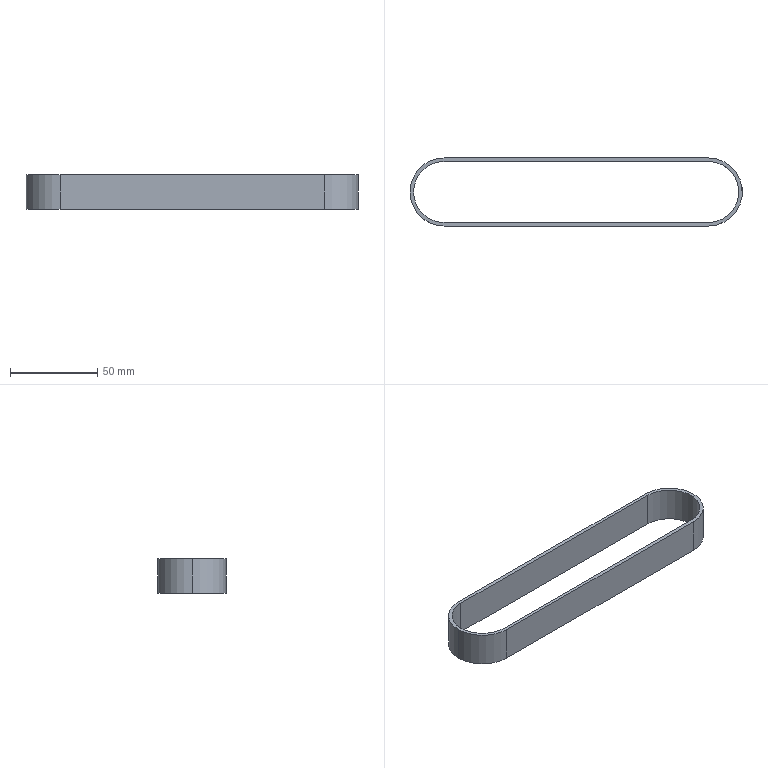Part | STEP file | Timing belt | 1 solid | 12 faces | box 190.16 x 39 x 20 mm | volume 16742 mm3 | cylinder 6 | plane 6 | commonest cylinder face diameters 35 x3 39 x3
STEP:
#1=CARTESIAN_POINT('',(0.,0.,0.));
#2=DIRECTION('',(0.,0.,1.));
#3=DIRECTION('',(1.,0.,0.));
#4=AXIS2_PLACEMENT_3D('',#1,#2,#3);
#5=CARTESIAN_POINT('',(-19.5,0.,20.));
#6=VERTEX_POINT('',#5);
#7=CARTESIAN_POINT('',(0.,-19.5,20.));
#8=VERTEX_POINT('',#7);
#9=CARTESIAN_POINT('',(0.,0.,20.));
#10=DIRECTION('',(0.,0.,1.));
#11=DIRECTION('',(-1.,0.,0.));
#12=AXIS2_PLACEMENT_3D('',#9,#10,#11);
#13=CIRCLE('',#12,19.5);
#14=CARTESIAN_POINT('',(0.,0.,20.));
#15=DIRECTION('',(0.,0.,-1.));
#16=DIRECTION('',(-1.,0.,0.));
#17=AXIS2_PLACEMENT_3D('',#14,#15,#16);
#18=CYLINDRICAL_SURFACE('',#17,19.5);
#19=CARTESIAN_POINT('',(6.283,0.));
#20=DIRECTION('',(-1.,0.));
#21=VECTOR('',#20,1.);
#22=LINE('',#19,#21);
#23=(GEOMETRIC_REPRESENTATION_CONTEXT(2)PARAMETRIC_REPRESENTATION_CONTEXT()REPRESENTATION_CONTEXT('',''));
#24=DEFINITIONAL_REPRESENTATION('',(#22),#23);
#25=PCURVE('',#18,#24);
#26=CARTESIAN_POINT('',(0.,0.,20.));
#27=DIRECTION('',(0.,0.,1.));
#28=DIRECTION('',(1.,0.,0.));
#29=AXIS2_PLACEMENT_3D('',#26,#27,#28);
#30=PLANE('',#29);
#31=CARTESIAN_POINT('',(0.,0.));
#32=DIRECTION('',(-1.,0.));
#33=AXIS2_PLACEMENT_2D('',#31,#32);
#34=CIRCLE('',#33,19.5);
#35=(GEOMETRIC_REPRESENTATION_CONTEXT(2)PARAMETRIC_REPRESENTATION_CONTEXT()REPRESENTATION_CONTEXT('',''));
#36=DEFINITIONAL_REPRESENTATION('',(#34),#35);
#37=PCURVE('',#30,#36);
#38=SURFACE_CURVE('',#13,(#25,#37),.PCURVE_S1.);
#39=EDGE_CURVE('',#6,#8,#38,.T.);
#40=ORIENTED_EDGE('',*,*,#39,.F.);
#41=CARTESIAN_POINT('',(-19.5,0.,0.));
#42=VERTEX_POINT('',#41);
#43=CARTESIAN_POINT('',(-19.5,0.,20.));
#44=DIRECTION('',(0.,0.,-1.));
#45=VECTOR('',#44,1.);
#46=LINE('',#43,#45);
#47=CARTESIAN_POINT('',(6.283,0.));
#48=DIRECTION('',(0.,1.));
#49=VECTOR('',#48,1.);
#50=LINE('',#47,#49);
#51=(GEOMETRIC_REPRESENTATION_CONTEXT(2)PARAMETRIC_REPRESENTATION_CONTEXT()REPRESENTATION_CONTEXT('',''));
#52=DEFINITIONAL_REPRESENTATION('',(#50),#51);
#53=PCURVE('',#18,#52);
#54=CARTESIAN_POINT('',(0.,0.,20.));
#55=DIRECTION('',(0.,0.,-1.));
#56=DIRECTION('',(-1.,0.,0.));
#57=AXIS2_PLACEMENT_3D('',#54,#55,#56);
#58=CYLINDRICAL_SURFACE('',#57,19.5);
#59=CARTESIAN_POINT('',(0.,0.));
#60=DIRECTION('',(0.,1.));
#61=VECTOR('',#60,1.);
#62=LINE('',#59,#61);
#63=(GEOMETRIC_REPRESENTATION_CONTEXT(2)PARAMETRIC_REPRESENTATION_CONTEXT()REPRESENTATION_CONTEXT('',''));
#64=DEFINITIONAL_REPRESENTATION('',(#62),#63);
#65=PCURVE('',#58,#64);
#66=SURFACE_CURVE('',#46,(#53,#65),.PCURVE_S1.);
#67=EDGE_CURVE('',#6,#42,#66,.T.);
#68=ORIENTED_EDGE('',*,*,#67,.T.);
#69=CARTESIAN_POINT('',(0.,-19.5,0.));
#70=VERTEX_POINT('',#69);
#71=CARTESIAN_POINT('',(0.,0.,0.));
#72=DIRECTION('',(0.,0.,1.));
#73=DIRECTION('',(-1.,0.,0.));
#74=AXIS2_PLACEMENT_3D('',#71,#72,#73);
#75=CIRCLE('',#74,19.5);
#76=CARTESIAN_POINT('',(6.283,20.));
#77=DIRECTION('',(-1.,0.));
#78=VECTOR('',#77,1.);
#79=LINE('',#76,#78);
#80=(GEOMETRIC_REPRESENTATION_CONTEXT(2)PARAMETRIC_REPRESENTATION_CONTEXT()REPRESENTATION_CONTEXT('',''));
#81=DEFINITIONAL_REPRESENTATION('',(#79),#80);
#82=PCURVE('',#18,#81);
#83=CARTESIAN_POINT('',(0.,0.,0.));
#84=DIRECTION('',(0.,0.,1.));
#85=DIRECTION('',(1.,0.,0.));
#86=AXIS2_PLACEMENT_3D('',#83,#84,#85);
#87=PLANE('',#86);
#88=CARTESIAN_POINT('',(0.,0.));
#89=DIRECTION('',(-1.,0.));
#90=AXIS2_PLACEMENT_2D('',#88,#89);
#91=CIRCLE('',#90,19.5);
#92=(GEOMETRIC_REPRESENTATION_CONTEXT(2)PARAMETRIC_REPRESENTATION_CONTEXT()REPRESENTATION_CONTEXT('',''));
#93=DEFINITIONAL_REPRESENTATION('',(#91),#92);
#94=PCURVE('',#87,#93);
#95=SURFACE_CURVE('',#75,(#82,#94),.PCURVE_S1.);
#96=EDGE_CURVE('',#42,#70,#95,.T.);
#97=ORIENTED_EDGE('',*,*,#96,.T.);
#98=CARTESIAN_POINT('',(0.,-19.5,20.));
#99=DIRECTION('',(0.,0.,1.));
#100=VECTOR('',#99,1.);
#101=LINE('',#98,#100);
#102=CARTESIAN_POINT('',(4.712,0.));
#103=DIRECTION('',(0.,-1.));
#104=VECTOR('',#103,1.);
#105=LINE('',#102,#104);
#106=(GEOMETRIC_REPRESENTATION_CONTEXT(2)PARAMETRIC_REPRESENTATION_CONTEXT()REPRESENTATION_CONTEXT('',''));
#107=DEFINITIONAL_REPRESENTATION('',(#105),#106);
#108=PCURVE('',#18,#107);
#109=CARTESIAN_POINT('',(0.,-19.5,20.));
#110=DIRECTION('',(0.,1.,0.));
#111=DIRECTION('',(0.,0.,1.));
#112=AXIS2_PLACEMENT_3D('',#109,#110,#111);
#113=PLANE('',#112);
#114=CARTESIAN_POINT('',(0.,0.));
#115=DIRECTION('',(1.,0.));
#116=VECTOR('',#115,1.);
#117=LINE('',#114,#116);
#118=(GEOMETRIC_REPRESENTATION_CONTEXT(2)PARAMETRIC_REPRESENTATION_CONTEXT()REPRESENTATION_CONTEXT('',''));
#119=DEFINITIONAL_REPRESENTATION('',(#117),#118);
#120=PCURVE('',#113,#119);
#121=SURFACE_CURVE('',#101,(#108,#120),.PCURVE_S1.);
#122=EDGE_CURVE('',#70,#8,#121,.T.);
#123=ORIENTED_EDGE('',*,*,#122,.T.);
#124=EDGE_LOOP('',(#40,#68,#97,#123));
#125=FACE_BOUND('',#124,.T.);
#126=ADVANCED_FACE('',(#125),#18,.T.);
#127=CARTESIAN_POINT('',(0.,17.5,20.));
#128=VERTEX_POINT('',#127);
#129=CARTESIAN_POINT('',(0.,17.5,0.));
#130=VERTEX_POINT('',#129);
#131=CARTESIAN_POINT('',(0.,17.5,20.));
#132=DIRECTION('',(0.,0.,-1.));
#133=VECTOR('',#132,1.);
#134=LINE('',#131,#133);
#135=CARTESIAN_POINT('',(0.,0.,20.));
#136=DIRECTION('',(0.,0.,-1.));
#137=DIRECTION('',(-1.,0.,0.));
#138=AXIS2_PLACEMENT_3D('',#135,#136,#137);
#139=CYLINDRICAL_SURFACE('',#138,17.5);
#140=CARTESIAN_POINT('',(1.571,0.));
#141=DIRECTION('',(0.,1.));
#142=VECTOR('',#141,1.);
#143=LINE('',#140,#142);
#144=(GEOMETRIC_REPRESENTATION_CONTEXT(2)PARAMETRIC_REPRESENTATION_CONTEXT()REPRESENTATION_CONTEXT('',''));
#145=DEFINITIONAL_REPRESENTATION('',(#143),#144);
#146=PCURVE('',#139,#145);
#147=CARTESIAN_POINT('',(0.,17.5,20.));
#148=DIRECTION('',(0.,-1.,0.));
#149=DIRECTION('',(0.,0.,-1.));
#150=AXIS2_PLACEMENT_3D('',#147,#148,#149);
#151=PLANE('',#150);
#152=CARTESIAN_POINT('',(0.,0.));
#153=DIRECTION('',(1.,0.));
#154=VECTOR('',#153,1.);
#155=LINE('',#152,#154);
#156=(GEOMETRIC_REPRESENTATION_CONTEXT(2)PARAMETRIC_REPRESENTATION_CONTEXT()REPRESENTATION_CONTEXT('',''));
#157=DEFINITIONAL_REPRESENTATION('',(#155),#156);
#158=PCURVE('',#151,#157);
#159=SURFACE_CURVE('',#134,(#146,#158),.PCURVE_S1.);
#160=EDGE_CURVE('',#128,#130,#159,.T.);
#161=ORIENTED_EDGE('',*,*,#160,.T.);
#162=CARTESIAN_POINT('',(-17.5,0.,0.));
#163=VERTEX_POINT('',#162);
#164=CARTESIAN_POINT('',(0.,0.,0.));
#165=DIRECTION('',(0.,0.,-1.));
#166=DIRECTION('',(-1.,0.,0.));
#167=AXIS2_PLACEMENT_3D('',#164,#165,#166);
#168=CIRCLE('',#167,17.5);
#169=CARTESIAN_POINT('',(0.,20.));
#170=DIRECTION('',(1.,0.));
#171=VECTOR('',#170,1.);
#172=LINE('',#169,#171);
#173=(GEOMETRIC_REPRESENTATION_CONTEXT(2)PARAMETRIC_REPRESENTATION_CONTEXT()REPRESENTATION_CONTEXT('',''));
#174=DEFINITIONAL_REPRESENTATION('',(#172),#173);
#175=PCURVE('',#139,#174);
#176=CARTESIAN_POINT('',(-17.5,0.));
#177=CARTESIAN_POINT('',(-17.5,30.311));
#178=CARTESIAN_POINT('',(8.75,15.155));
#179=CARTESIAN_POINT('',(35.,0.));
#180=CARTESIAN_POINT('',(8.75,-15.155));
#181=CARTESIAN_POINT('',(-17.5,-30.311));
#182=CARTESIAN_POINT('',(-17.5,0.));
#183=(BOUNDED_CURVE()B_SPLINE_CURVE(2,(#176,#177,#178,#179,#180,#181,#182),.UNSPECIFIED.,.T.,.F.)B_SPLINE_CURVE_WITH_KNOTS((1,2,2,2,2,1),(-2.094,0.,2.094,4.189,6.283,8.378),.UNSPECIFIED.)CURVE()GEOMETRIC_REPRESENTATION_ITEM()RATIONAL_B_SPLINE_CURVE((1.,0.5,1.,0.5,1.,0.5,1.))REPRESENTATION_ITEM(''));
#184=(GEOMETRIC_REPRESENTATION_CONTEXT(2)PARAMETRIC_REPRESENTATION_CONTEXT()REPRESENTATION_CONTEXT('',''));
#185=DEFINITIONAL_REPRESENTATION('',(#183),#184);
#186=PCURVE('',#87,#185);
#187=SURFACE_CURVE('',#168,(#175,#186),.PCURVE_S1.);
#188=EDGE_CURVE('',#163,#130,#187,.T.);
#189=ORIENTED_EDGE('',*,*,#188,.F.);
#190=CARTESIAN_POINT('',(-17.5,0.,20.));
#191=VERTEX_POINT('',#190);
#192=CARTESIAN_POINT('',(-17.5,0.,20.));
#193=DIRECTION('',(0.,0.,-1.));
#194=VECTOR('',#193,1.);
#195=LINE('',#192,#194);
#196=CARTESIAN_POINT('',(0.,0.));
#197=DIRECTION('',(0.,1.));
#198=VECTOR('',#197,1.);
#199=LINE('',#196,#198);
#200=(GEOMETRIC_REPRESENTATION_CONTEXT(2)PARAMETRIC_REPRESENTATION_CONTEXT()REPRESENTATION_CONTEXT('',''));
#201=DEFINITIONAL_REPRESENTATION('',(#199),#200);
#202=PCURVE('',#139,#201);
#203=CARTESIAN_POINT('',(0.,0.,20.));
#204=DIRECTION('',(0.,0.,-1.));
#205=DIRECTION('',(-1.,0.,0.));
#206=AXIS2_PLACEMENT_3D('',#203,#204,#205);
#207=CYLINDRICAL_SURFACE('',#206,17.5);
#208=CARTESIAN_POINT('',(6.283,0.));
#209=DIRECTION('',(0.,1.));
#210=VECTOR('',#209,1.);
#211=LINE('',#208,#210);
#212=(GEOMETRIC_REPRESENTATION_CONTEXT(2)PARAMETRIC_REPRESENTATION_CONTEXT()REPRESENTATION_CONTEXT('',''));
#213=DEFINITIONAL_REPRESENTATION('',(#211),#212);
#214=PCURVE('',#207,#213);
#215=SURFACE_CURVE('',#195,(#202,#214),.PCURVE_S1.);
#216=EDGE_CURVE('',#191,#163,#215,.T.);
#217=ORIENTED_EDGE('',*,*,#216,.F.);
#218=CARTESIAN_POINT('',(0.,0.,20.));
#219=DIRECTION('',(0.,0.,-1.));
#220=DIRECTION('',(-1.,0.,0.));
#221=AXIS2_PLACEMENT_3D('',#218,#219,#220);
#222=CIRCLE('',#221,17.5);
#223=CARTESIAN_POINT('',(0.,0.));
#224=DIRECTION('',(1.,0.));
#225=VECTOR('',#224,1.);
#226=LINE('',#223,#225);
#227=(GEOMETRIC_REPRESENTATION_CONTEXT(2)PARAMETRIC_REPRESENTATION_CONTEXT()REPRESENTATION_CONTEXT('',''));
#228=DEFINITIONAL_REPRESENTATION('',(#226),#227);
#229=PCURVE('',#139,#228);
#230=CARTESIAN_POINT('',(-17.5,0.));
#231=CARTESIAN_POINT('',(-17.5,30.311));
#232=CARTESIAN_POINT('',(8.75,15.155));
#233=CARTESIAN_POINT('',(35.,0.));
#234=CARTESIAN_POINT('',(8.75,-15.155));
#235=CARTESIAN_POINT('',(-17.5,-30.311));
#236=CARTESIAN_POINT('',(-17.5,0.));
#237=(BOUNDED_CURVE()B_SPLINE_CURVE(2,(#230,#231,#232,#233,#234,#235,#236),.UNSPECIFIED.,.T.,.F.)B_SPLINE_CURVE_WITH_KNOTS((1,2,2,2,2,1),(-2.094,0.,2.094,4.189,6.283,8.378),.UNSPECIFIED.)CURVE()GEOMETRIC_REPRESENTATION_ITEM()RATIONAL_B_SPLINE_CURVE((1.,0.5,1.,0.5,1.,0.5,1.))REPRESENTATION_ITEM(''));
#238=(GEOMETRIC_REPRESENTATION_CONTEXT(2)PARAMETRIC_REPRESENTATION_CONTEXT()REPRESENTATION_CONTEXT('',''));
#239=DEFINITIONAL_REPRESENTATION('',(#237),#238);
#240=PCURVE('',#30,#239);
#241=SURFACE_CURVE('',#222,(#229,#240),.PCURVE_S1.);
#242=EDGE_CURVE('',#191,#128,#241,.T.);
#243=ORIENTED_EDGE('',*,*,#242,.T.);
#244=EDGE_LOOP('',(#161,#189,#217,#243));
#245=FACE_BOUND('',#244,.F.);
#246=ADVANCED_FACE('',(#245),#139,.F.);
#247=CARTESIAN_POINT('',(151.16,-19.5,20.));
#248=VERTEX_POINT('',#247);
#249=CARTESIAN_POINT('',(151.16,-19.5,0.));
#250=VERTEX_POINT('',#249);
#251=CARTESIAN_POINT('',(151.16,-19.5,20.));
#252=DIRECTION('',(0.,0.,-1.));
#253=VECTOR('',#252,1.);
#254=LINE('',#251,#253);
#255=CARTESIAN_POINT('',(0.,151.16));
#256=DIRECTION('',(-1.,0.));
#257=VECTOR('',#256,1.);
#258=LINE('',#255,#257);
#259=(GEOMETRIC_REPRESENTATION_CONTEXT(2)PARAMETRIC_REPRESENTATION_CONTEXT()REPRESENTATION_CONTEXT('',''));
#260=DEFINITIONAL_REPRESENTATION('',(#258),#259);
#261=PCURVE('',#113,#260);
#262=CARTESIAN_POINT('',(151.16,0.,20.));
#263=DIRECTION('',(0.,0.,-1.));
#264=DIRECTION('',(-1.,0.,0.));
#265=AXIS2_PLACEMENT_3D('',#262,#263,#264);
#266=CYLINDRICAL_SURFACE('',#265,19.5);
#267=CARTESIAN_POINT('',(4.712,0.));
#268=DIRECTION('',(0.,1.));
#269=VECTOR('',#268,1.);
#270=LINE('',#267,#269);
#271=(GEOMETRIC_REPRESENTATION_CONTEXT(2)PARAMETRIC_REPRESENTATION_CONTEXT()REPRESENTATION_CONTEXT('',''));
#272=DEFINITIONAL_REPRESENTATION('',(#270),#271);
#273=PCURVE('',#266,#272);
#274=SURFACE_CURVE('',#254,(#261,#273),.PCURVE_S1.);
#275=EDGE_CURVE('',#248,#250,#274,.T.);
#276=ORIENTED_EDGE('',*,*,#275,.F.);
#277=CARTESIAN_POINT('',(0.,-19.5,20.));
#278=DIRECTION('',(1.,0.,0.));
#279=VECTOR('',#278,1.);
#280=LINE('',#277,#279);
#281=CARTESIAN_POINT('',(0.,0.));
#282=DIRECTION('',(0.,1.));
#283=VECTOR('',#282,1.);
#284=LINE('',#281,#283);
#285=(GEOMETRIC_REPRESENTATION_CONTEXT(2)PARAMETRIC_REPRESENTATION_CONTEXT()REPRESENTATION_CONTEXT('',''));
#286=DEFINITIONAL_REPRESENTATION('',(#284),#285);
#287=PCURVE('',#113,#286);
#288=CARTESIAN_POINT('',(0.,-19.5));
#289=DIRECTION('',(1.,0.));
#290=VECTOR('',#289,1.);
#291=LINE('',#288,#290);
#292=(GEOMETRIC_REPRESENTATION_CONTEXT(2)PARAMETRIC_REPRESENTATION_CONTEXT()REPRESENTATION_CONTEXT('',''));
#293=DEFINITIONAL_REPRESENTATION('',(#291),#292);
#294=PCURVE('',#30,#293);
#295=SURFACE_CURVE('',#280,(#287,#294),.PCURVE_S1.);
#296=EDGE_CURVE('',#8,#248,#295,.T.);
#297=ORIENTED_EDGE('',*,*,#296,.F.);
#298=ORIENTED_EDGE('',*,*,#122,.F.);
#299=CARTESIAN_POINT('',(0.,-19.5,0.));
#300=DIRECTION('',(-1.,0.,0.));
#301=VECTOR('',#300,1.);
#302=LINE('',#299,#301);
#303=CARTESIAN_POINT('',(-20.,0.));
#304=DIRECTION('',(0.,-1.));
#305=VECTOR('',#304,1.);
#306=LINE('',#303,#305);
#307=(GEOMETRIC_REPRESENTATION_CONTEXT(2)PARAMETRIC_REPRESENTATION_CONTEXT()REPRESENTATION_CONTEXT('',''));
#308=DEFINITIONAL_REPRESENTATION('',(#306),#307);
#309=PCURVE('',#113,#308);
#310=CARTESIAN_POINT('',(0.,-19.5));
#311=DIRECTION('',(-1.,0.));
#312=VECTOR('',#311,1.);
#313=LINE('',#310,#312);
#314=(GEOMETRIC_REPRESENTATION_CONTEXT(2)PARAMETRIC_REPRESENTATION_CONTEXT()REPRESENTATION_CONTEXT('',''));
#315=DEFINITIONAL_REPRESENTATION('',(#313),#314);
#316=PCURVE('',#87,#315);
#317=SURFACE_CURVE('',#302,(#309,#316),.PCURVE_S1.);
#318=EDGE_CURVE('',#250,#70,#317,.T.);
#319=ORIENTED_EDGE('',*,*,#318,.F.);
#320=EDGE_LOOP('',(#276,#297,#298,#319));
#321=FACE_BOUND('',#320,.T.);
#322=ADVANCED_FACE('',(#321),#113,.F.);
#323=CARTESIAN_POINT('',(0.,-17.5,0.));
#324=VERTEX_POINT('',#323);
#325=CARTESIAN_POINT('',(0.,0.,0.));
#326=DIRECTION('',(0.,0.,-1.));
#327=DIRECTION('',(-1.,0.,0.));
#328=AXIS2_PLACEMENT_3D('',#325,#326,#327);
#329=CIRCLE('',#328,17.5);
#330=CARTESIAN_POINT('',(-17.5,0.));
#331=CARTESIAN_POINT('',(-17.5,30.311));
#332=CARTESIAN_POINT('',(8.75,15.155));
#333=CARTESIAN_POINT('',(35.,0.));
#334=CARTESIAN_POINT('',(8.75,-15.155));
#335=CARTESIAN_POINT('',(-17.5,-30.311));
#336=CARTESIAN_POINT('',(-17.5,0.));
#337=(BOUNDED_CURVE()B_SPLINE_CURVE(2,(#330,#331,#332,#333,#334,#335,#336),.UNSPECIFIED.,.T.,.F.)B_SPLINE_CURVE_WITH_KNOTS((1,2,2,2,2,1),(-2.094,0.,2.094,4.189,6.283,8.378),.UNSPECIFIED.)CURVE()GEOMETRIC_REPRESENTATION_ITEM()RATIONAL_B_SPLINE_CURVE((1.,0.5,1.,0.5,1.,0.5,1.))REPRESENTATION_ITEM(''));
#338=(GEOMETRIC_REPRESENTATION_CONTEXT(2)PARAMETRIC_REPRESENTATION_CONTEXT()REPRESENTATION_CONTEXT('',''));
#339=DEFINITIONAL_REPRESENTATION('',(#337),#338);
#340=PCURVE('',#87,#339);
#341=CARTESIAN_POINT('',(0.,20.));
#342=DIRECTION('',(1.,0.));
#343=VECTOR('',#342,1.);
#344=LINE('',#341,#343);
#345=(GEOMETRIC_REPRESENTATION_CONTEXT(2)PARAMETRIC_REPRESENTATION_CONTEXT()REPRESENTATION_CONTEXT('',''));
#346=DEFINITIONAL_REPRESENTATION('',(#344),#345);
#347=PCURVE('',#207,#346);
#348=SURFACE_CURVE('',#329,(#340,#347),.PCURVE_S1.);
#349=EDGE_CURVE('',#324,#163,#348,.T.);
#350=ORIENTED_EDGE('',*,*,#349,.F.);
#351=CARTESIAN_POINT('',(151.16,-17.5,0.));
#352=VERTEX_POINT('',#351);
#353=CARTESIAN_POINT('',(0.,-17.5,0.));
#354=DIRECTION('',(-1.,0.,0.));
#355=VECTOR('',#354,1.);
#356=LINE('',#353,#355);
#357=CARTESIAN_POINT('',(0.,-17.5));
#358=DIRECTION('',(-1.,0.));
#359=VECTOR('',#358,1.);
#360=LINE('',#357,#359);
#361=(GEOMETRIC_REPRESENTATION_CONTEXT(2)PARAMETRIC_REPRESENTATION_CONTEXT()REPRESENTATION_CONTEXT('',''));
#362=DEFINITIONAL_REPRESENTATION('',(#360),#361);
#363=PCURVE('',#87,#362);
#364=CARTESIAN_POINT('',(0.,-17.5,20.));
#365=DIRECTION('',(0.,1.,0.));
#366=DIRECTION('',(0.,0.,1.));
#367=AXIS2_PLACEMENT_3D('',#364,#365,#366);
#368=PLANE('',#367);
#369=CARTESIAN_POINT('',(-20.,0.));
#370=DIRECTION('',(0.,-1.));
#371=VECTOR('',#370,1.);
#372=LINE('',#369,#371);
#373=(GEOMETRIC_REPRESENTATION_CONTEXT(2)PARAMETRIC_REPRESENTATION_CONTEXT()REPRESENTATION_CONTEXT('',''));
#374=DEFINITIONAL_REPRESENTATION('',(#372),#373);
#375=PCURVE('',#368,#374);
#376=SURFACE_CURVE('',#356,(#363,#375),.PCURVE_S1.);
#377=EDGE_CURVE('',#352,#324,#376,.T.);
#378=ORIENTED_EDGE('',*,*,#377,.F.);
#379=CARTESIAN_POINT('',(151.16,17.5,0.));
#380=VERTEX_POINT('',#379);
#381=CARTESIAN_POINT('',(151.16,0.,0.));
#382=DIRECTION('',(0.,0.,-1.));
#383=DIRECTION('',(-1.,0.,0.));
#384=AXIS2_PLACEMENT_3D('',#381,#382,#383);
#385=CIRCLE('',#384,17.5);
#386=CARTESIAN_POINT('',(133.66,0.));
#387=CARTESIAN_POINT('',(133.66,30.311));
#388=CARTESIAN_POINT('',(159.91,15.155));
#389=CARTESIAN_POINT('',(186.16,0.));
#390=CARTESIAN_POINT('',(159.91,-15.155));
#391=CARTESIAN_POINT('',(133.66,-30.311));
#392=CARTESIAN_POINT('',(133.66,0.));
#393=(BOUNDED_CURVE()B_SPLINE_CURVE(2,(#386,#387,#388,#389,#390,#391,#392),.UNSPECIFIED.,.T.,.F.)B_SPLINE_CURVE_WITH_KNOTS((1,2,2,2,2,1),(-2.094,0.,2.094,4.189,6.283,8.378),.UNSPECIFIED.)CURVE()GEOMETRIC_REPRESENTATION_ITEM()RATIONAL_B_SPLINE_CURVE((1.,0.5,1.,0.5,1.,0.5,1.))REPRESENTATION_ITEM(''));
#394=(GEOMETRIC_REPRESENTATION_CONTEXT(2)PARAMETRIC_REPRESENTATION_CONTEXT()REPRESENTATION_CONTEXT('',''));
#395=DEFINITIONAL_REPRESENTATION('',(#393),#394);
#396=PCURVE('',#87,#395);
#397=CARTESIAN_POINT('',(151.16,0.,20.));
#398=DIRECTION('',(0.,0.,-1.));
#399=DIRECTION('',(-1.,0.,0.));
#400=AXIS2_PLACEMENT_3D('',#397,#398,#399);
#401=CYLINDRICAL_SURFACE('',#400,17.5);
#402=CARTESIAN_POINT('',(0.,20.));
#403=DIRECTION('',(1.,0.));
#404=VECTOR('',#403,1.);
#405=LINE('',#402,#404);
#406=(GEOMETRIC_REPRESENTATION_CONTEXT(2)PARAMETRIC_REPRESENTATION_CONTEXT()REPRESENTATION_CONTEXT('',''));
#407=DEFINITIONAL_REPRESENTATION('',(#405),#406);
#408=PCURVE('',#401,#407);
#409=SURFACE_CURVE('',#385,(#396,#408),.PCURVE_S1.);
#410=EDGE_CURVE('',#380,#352,#409,.T.);
#411=ORIENTED_EDGE('',*,*,#410,.F.);
#412=CARTESIAN_POINT('',(0.,17.5,0.));
#413=DIRECTION('',(1.,0.,0.));
#414=VECTOR('',#413,1.);
#415=LINE('',#412,#414);
#416=CARTESIAN_POINT('',(0.,17.5));
#417=DIRECTION('',(1.,0.));
#418=VECTOR('',#417,1.);
#419=LINE('',#416,#418);
#420=(GEOMETRIC_REPRESENTATION_CONTEXT(2)PARAMETRIC_REPRESENTATION_CONTEXT()REPRESENTATION_CONTEXT('',''));
#421=DEFINITIONAL_REPRESENTATION('',(#419),#420);
#422=PCURVE('',#87,#421);
#423=CARTESIAN_POINT('',(20.,0.));
#424=DIRECTION('',(0.,1.));
#425=VECTOR('',#424,1.);
#426=LINE('',#423,#425);
#427=(GEOMETRIC_REPRESENTATION_CONTEXT(2)PARAMETRIC_REPRESENTATION_CONTEXT()REPRESENTATION_CONTEXT('',''));
#428=DEFINITIONAL_REPRESENTATION('',(#426),#427);
#429=PCURVE('',#151,#428);
#430=SURFACE_CURVE('',#415,(#422,#429),.PCURVE_S1.);
#431=EDGE_CURVE('',#130,#380,#430,.T.);
#432=ORIENTED_EDGE('',*,*,#431,.F.);
#433=ORIENTED_EDGE('',*,*,#188,.F.);
#434=EDGE_LOOP('',(#350,#378,#411,#432,#433));
#435=FACE_BOUND('',#434,.T.);
#436=CARTESIAN_POINT('',(151.16,19.5,0.));
#437=VERTEX_POINT('',#436);
#438=CARTESIAN_POINT('',(0.,19.5,0.));
#439=VERTEX_POINT('',#438);
#440=CARTESIAN_POINT('',(0.,19.5,0.));
#441=DIRECTION('',(-1.,0.,0.));
#442=VECTOR('',#441,1.);
#443=LINE('',#440,#442);
#444=CARTESIAN_POINT('',(0.,19.5));
#445=DIRECTION('',(-1.,0.));
#446=VECTOR('',#445,1.);
#447=LINE('',#444,#446);
#448=(GEOMETRIC_REPRESENTATION_CONTEXT(2)PARAMETRIC_REPRESENTATION_CONTEXT()REPRESENTATION_CONTEXT('',''));
#449=DEFINITIONAL_REPRESENTATION('',(#447),#448);
#450=PCURVE('',#87,#449);
#451=CARTESIAN_POINT('',(0.,19.5,20.));
#452=DIRECTION('',(0.,-1.,0.));
#453=DIRECTION('',(0.,0.,-1.));
#454=AXIS2_PLACEMENT_3D('',#451,#452,#453);
#455=PLANE('',#454);
#456=CARTESIAN_POINT('',(20.,0.));
#457=DIRECTION('',(0.,-1.));
#458=VECTOR('',#457,1.);
#459=LINE('',#456,#458);
#460=(GEOMETRIC_REPRESENTATION_CONTEXT(2)PARAMETRIC_REPRESENTATION_CONTEXT()REPRESENTATION_CONTEXT('',''));
#461=DEFINITIONAL_REPRESENTATION('',(#459),#460);
#462=PCURVE('',#455,#461);
#463=SURFACE_CURVE('',#443,(#450,#462),.PCURVE_S1.);
#464=EDGE_CURVE('',#437,#439,#463,.T.);
#465=ORIENTED_EDGE('',*,*,#464,.F.);
#466=CARTESIAN_POINT('',(151.16,0.,0.));
#467=DIRECTION('',(0.,0.,1.));
#468=DIRECTION('',(-1.,0.,0.));
#469=AXIS2_PLACEMENT_3D('',#466,#467,#468);
#470=CIRCLE('',#469,19.5);
#471=CARTESIAN_POINT('',(151.16,0.));
#472=DIRECTION('',(-1.,0.));
#473=AXIS2_PLACEMENT_2D('',#471,#472);
#474=CIRCLE('',#473,19.5);
#475=(GEOMETRIC_REPRESENTATION_CONTEXT(2)PARAMETRIC_REPRESENTATION_CONTEXT()REPRESENTATION_CONTEXT('',''));
#476=DEFINITIONAL_REPRESENTATION('',(#474),#475);
#477=PCURVE('',#87,#476);
#478=CARTESIAN_POINT('',(6.283,20.));
#479=DIRECTION('',(-1.,0.));
#480=VECTOR('',#479,1.);
#481=LINE('',#478,#480);
#482=(GEOMETRIC_REPRESENTATION_CONTEXT(2)PARAMETRIC_REPRESENTATION_CONTEXT()REPRESENTATION_CONTEXT('',''));
#483=DEFINITIONAL_REPRESENTATION('',(#481),#482);
#484=PCURVE('',#266,#483);
#485=SURFACE_CURVE('',#470,(#477,#484),.PCURVE_S1.);
#486=EDGE_CURVE('',#250,#437,#485,.T.);
#487=ORIENTED_EDGE('',*,*,#486,.F.);
#488=ORIENTED_EDGE('',*,*,#318,.T.);
#489=ORIENTED_EDGE('',*,*,#96,.F.);
#490=CARTESIAN_POINT('',(0.,0.,0.));
#491=DIRECTION('',(0.,0.,1.));
#492=DIRECTION('',(-1.,0.,0.));
#493=AXIS2_PLACEMENT_3D('',#490,#491,#492);
#494=CIRCLE('',#493,19.5);
#495=CARTESIAN_POINT('',(0.,0.));
#496=DIRECTION('',(-1.,0.));
#497=AXIS2_PLACEMENT_2D('',#495,#496);
#498=CIRCLE('',#497,19.5);
#499=(GEOMETRIC_REPRESENTATION_CONTEXT(2)PARAMETRIC_REPRESENTATION_CONTEXT()REPRESENTATION_CONTEXT('',''));
#500=DEFINITIONAL_REPRESENTATION('',(#498),#499);
#501=PCURVE('',#87,#500);
#502=CARTESIAN_POINT('',(6.283,20.));
#503=DIRECTION('',(-1.,0.));
#504=VECTOR('',#503,1.);
#505=LINE('',#502,#504);
#506=(GEOMETRIC_REPRESENTATION_CONTEXT(2)PARAMETRIC_REPRESENTATION_CONTEXT()REPRESENTATION_CONTEXT('',''));
#507=DEFINITIONAL_REPRESENTATION('',(#505),#506);
#508=PCURVE('',#58,#507);
#509=SURFACE_CURVE('',#494,(#501,#508),.PCURVE_S1.);
#510=EDGE_CURVE('',#439,#42,#509,.T.);
#511=ORIENTED_EDGE('',*,*,#510,.F.);
#512=EDGE_LOOP('',(#465,#487,#488,#489,#511));
#513=FACE_BOUND('',#512,.T.);
#514=ADVANCED_FACE('',(#435,#513),#87,.F.);
#515=CARTESIAN_POINT('',(151.16,19.5,20.));
#516=VERTEX_POINT('',#515);
#517=CARTESIAN_POINT('',(151.16,0.,20.));
#518=DIRECTION('',(0.,0.,-1.));
#519=DIRECTION('',(-1.,0.,0.));
#520=AXIS2_PLACEMENT_3D('',#517,#518,#519);
#521=CIRCLE('',#520,19.5);
#522=CARTESIAN_POINT('',(0.,0.));
#523=DIRECTION('',(1.,0.));
#524=VECTOR('',#523,1.);
#525=LINE('',#522,#524);
#526=(GEOMETRIC_REPRESENTATION_CONTEXT(2)PARAMETRIC_REPRESENTATION_CONTEXT()REPRESENTATION_CONTEXT('',''));
#527=DEFINITIONAL_REPRESENTATION('',(#525),#526);
#528=PCURVE('',#266,#527);
#529=CARTESIAN_POINT('',(131.66,0.));
#530=CARTESIAN_POINT('',(131.66,33.775));
#531=CARTESIAN_POINT('',(160.91,16.887));
#532=CARTESIAN_POINT('',(190.16,0.));
#533=CARTESIAN_POINT('',(160.91,-16.887));
#534=CARTESIAN_POINT('',(131.66,-33.775));
#535=CARTESIAN_POINT('',(131.66,0.));
#536=(BOUNDED_CURVE()B_SPLINE_CURVE(2,(#529,#530,#531,#532,#533,#534,#535),.UNSPECIFIED.,.T.,.F.)B_SPLINE_CURVE_WITH_KNOTS((1,2,2,2,2,1),(-2.094,0.,2.094,4.189,6.283,8.378),.UNSPECIFIED.)CURVE()GEOMETRIC_REPRESENTATION_ITEM()RATIONAL_B_SPLINE_CURVE((1.,0.5,1.,0.5,1.,0.5,1.))REPRESENTATION_ITEM(''));
#537=(GEOMETRIC_REPRESENTATION_CONTEXT(2)PARAMETRIC_REPRESENTATION_CONTEXT()REPRESENTATION_CONTEXT('',''));
#538=DEFINITIONAL_REPRESENTATION('',(#536),#537);
#539=PCURVE('',#30,#538);
#540=SURFACE_CURVE('',#521,(#528,#539),.PCURVE_S1.);
#541=EDGE_CURVE('',#516,#248,#540,.T.);
#542=ORIENTED_EDGE('',*,*,#541,.T.);
#543=ORIENTED_EDGE('',*,*,#275,.T.);
#544=ORIENTED_EDGE('',*,*,#486,.T.);
#545=CARTESIAN_POINT('',(151.16,19.5,20.));
#546=DIRECTION('',(0.,0.,1.));
#547=VECTOR('',#546,1.);
#548=LINE('',#545,#547);
#549=CARTESIAN_POINT('',(1.571,0.));
#550=DIRECTION('',(0.,-1.));
#551=VECTOR('',#550,1.);
#552=LINE('',#549,#551);
#553=(GEOMETRIC_REPRESENTATION_CONTEXT(2)PARAMETRIC_REPRESENTATION_CONTEXT()REPRESENTATION_CONTEXT('',''));
#554=DEFINITIONAL_REPRESENTATION('',(#552),#553);
#555=PCURVE('',#266,#554);
#556=CARTESIAN_POINT('',(0.,151.16));
#557=DIRECTION('',(-1.,0.));
#558=VECTOR('',#557,1.);
#559=LINE('',#556,#558);
#560=(GEOMETRIC_REPRESENTATION_CONTEXT(2)PARAMETRIC_REPRESENTATION_CONTEXT()REPRESENTATION_CONTEXT('',''));
#561=DEFINITIONAL_REPRESENTATION('',(#559),#560);
#562=PCURVE('',#455,#561);
#563=SURFACE_CURVE('',#548,(#555,#562),.PCURVE_S1.);
#564=EDGE_CURVE('',#437,#516,#563,.T.);
#565=ORIENTED_EDGE('',*,*,#564,.T.);
#566=EDGE_LOOP('',(#542,#543,#544,#565));
#567=FACE_BOUND('',#566,.T.);
#568=ADVANCED_FACE('',(#567),#266,.T.);
#569=CARTESIAN_POINT('',(151.16,17.5,20.));
#570=VERTEX_POINT('',#569);
#571=CARTESIAN_POINT('',(0.,17.5,20.));
#572=DIRECTION('',(1.,0.,0.));
#573=VECTOR('',#572,1.);
#574=LINE('',#571,#573);
#575=CARTESIAN_POINT('',(0.,17.5));
#576=DIRECTION('',(1.,0.));
#577=VECTOR('',#576,1.);
#578=LINE('',#575,#577);
#579=(GEOMETRIC_REPRESENTATION_CONTEXT(2)PARAMETRIC_REPRESENTATION_CONTEXT()REPRESENTATION_CONTEXT('',''));
#580=DEFINITIONAL_REPRESENTATION('',(#578),#579);
#581=PCURVE('',#30,#580);
#582=CARTESIAN_POINT('',(0.,0.));
#583=DIRECTION('',(0.,1.));
#584=VECTOR('',#583,1.);
#585=LINE('',#582,#584);
#586=(GEOMETRIC_REPRESENTATION_CONTEXT(2)PARAMETRIC_REPRESENTATION_CONTEXT()REPRESENTATION_CONTEXT('',''));
#587=DEFINITIONAL_REPRESENTATION('',(#585),#586);
#588=PCURVE('',#151,#587);
#589=SURFACE_CURVE('',#574,(#581,#588),.PCURVE_S1.);
#590=EDGE_CURVE('',#128,#570,#589,.T.);
#591=ORIENTED_EDGE('',*,*,#590,.T.);
#592=CARTESIAN_POINT('',(151.16,-17.5,20.));
#593=VERTEX_POINT('',#592);
#594=CARTESIAN_POINT('',(151.16,0.,20.));
#595=DIRECTION('',(0.,0.,-1.));
#596=DIRECTION('',(-1.,0.,0.));
#597=AXIS2_PLACEMENT_3D('',#594,#595,#596);
#598=CIRCLE('',#597,17.5);
#599=CARTESIAN_POINT('',(133.66,0.));
#600=CARTESIAN_POINT('',(133.66,30.311));
#601=CARTESIAN_POINT('',(159.91,15.155));
#602=CARTESIAN_POINT('',(186.16,0.));
#603=CARTESIAN_POINT('',(159.91,-15.155));
#604=CARTESIAN_POINT('',(133.66,-30.311));
#605=CARTESIAN_POINT('',(133.66,0.));
#606=(BOUNDED_CURVE()B_SPLINE_CURVE(2,(#599,#600,#601,#602,#603,#604,#605),.UNSPECIFIED.,.T.,.F.)B_SPLINE_CURVE_WITH_KNOTS((1,2,2,2,2,1),(-2.094,0.,2.094,4.189,6.283,8.378),.UNSPECIFIED.)CURVE()GEOMETRIC_REPRESENTATION_ITEM()RATIONAL_B_SPLINE_CURVE((1.,0.5,1.,0.5,1.,0.5,1.))REPRESENTATION_ITEM(''));
#607=(GEOMETRIC_REPRESENTATION_CONTEXT(2)PARAMETRIC_REPRESENTATION_CONTEXT()REPRESENTATION_CONTEXT('',''));
#608=DEFINITIONAL_REPRESENTATION('',(#606),#607);
#609=PCURVE('',#30,#608);
#610=CARTESIAN_POINT('',(0.,0.));
#611=DIRECTION('',(1.,0.));
#612=VECTOR('',#611,1.);
#613=LINE('',#610,#612);
#614=(GEOMETRIC_REPRESENTATION_CONTEXT(2)PARAMETRIC_REPRESENTATION_CONTEXT()REPRESENTATION_CONTEXT('',''));
#615=DEFINITIONAL_REPRESENTATION('',(#613),#614);
#616=PCURVE('',#401,#615);
#617=SURFACE_CURVE('',#598,(#609,#616),.PCURVE_S1.);
#618=EDGE_CURVE('',#570,#593,#617,.T.);
#619=ORIENTED_EDGE('',*,*,#618,.T.);
#620=CARTESIAN_POINT('',(0.,-17.5,20.));
#621=VERTEX_POINT('',#620);
#622=CARTESIAN_POINT('',(0.,-17.5,20.));
#623=DIRECTION('',(-1.,0.,0.));
#624=VECTOR('',#623,1.);
#625=LINE('',#622,#624);
#626=CARTESIAN_POINT('',(0.,-17.5));
#627=DIRECTION('',(-1.,0.));
#628=VECTOR('',#627,1.);
#629=LINE('',#626,#628);
#630=(GEOMETRIC_REPRESENTATION_CONTEXT(2)PARAMETRIC_REPRESENTATION_CONTEXT()REPRESENTATION_CONTEXT('',''));
#631=DEFINITIONAL_REPRESENTATION('',(#629),#630);
#632=PCURVE('',#30,#631);
#633=CARTESIAN_POINT('',(0.,0.));
#634=DIRECTION('',(0.,-1.));
#635=VECTOR('',#634,1.);
#636=LINE('',#633,#635);
#637=(GEOMETRIC_REPRESENTATION_CONTEXT(2)PARAMETRIC_REPRESENTATION_CONTEXT()REPRESENTATION_CONTEXT('',''));
#638=DEFINITIONAL_REPRESENTATION('',(#636),#637);
#639=PCURVE('',#368,#638);
#640=SURFACE_CURVE('',#625,(#632,#639),.PCURVE_S1.);
#641=EDGE_CURVE('',#593,#621,#640,.T.);
#642=ORIENTED_EDGE('',*,*,#641,.T.);
#643=CARTESIAN_POINT('',(0.,0.,20.));
#644=DIRECTION('',(0.,0.,-1.));
#645=DIRECTION('',(-1.,0.,0.));
#646=AXIS2_PLACEMENT_3D('',#643,#644,#645);
#647=CIRCLE('',#646,17.5);
#648=CARTESIAN_POINT('',(-17.5,0.));
#649=CARTESIAN_POINT('',(-17.5,30.311));
#650=CARTESIAN_POINT('',(8.75,15.155));
#651=CARTESIAN_POINT('',(35.,0.));
#652=CARTESIAN_POINT('',(8.75,-15.155));
#653=CARTESIAN_POINT('',(-17.5,-30.311));
#654=CARTESIAN_POINT('',(-17.5,0.));
#655=(BOUNDED_CURVE()B_SPLINE_CURVE(2,(#648,#649,#650,#651,#652,#653,#654),.UNSPECIFIED.,.T.,.F.)B_SPLINE_CURVE_WITH_KNOTS((1,2,2,2,2,1),(-2.094,0.,2.094,4.189,6.283,8.378),.UNSPECIFIED.)CURVE()GEOMETRIC_REPRESENTATION_ITEM()RATIONAL_B_SPLINE_CURVE((1.,0.5,1.,0.5,1.,0.5,1.))REPRESENTATION_ITEM(''));
#656=(GEOMETRIC_REPRESENTATION_CONTEXT(2)PARAMETRIC_REPRESENTATION_CONTEXT()REPRESENTATION_CONTEXT('',''));
#657=DEFINITIONAL_REPRESENTATION('',(#655),#656);
#658=PCURVE('',#30,#657);
#659=CARTESIAN_POINT('',(0.,0.));
#660=DIRECTION('',(1.,0.));
#661=VECTOR('',#660,1.);
#662=LINE('',#659,#661);
#663=(GEOMETRIC_REPRESENTATION_CONTEXT(2)PARAMETRIC_REPRESENTATION_CONTEXT()REPRESENTATION_CONTEXT('',''));
#664=DEFINITIONAL_REPRESENTATION('',(#662),#663);
#665=PCURVE('',#207,#664);
#666=SURFACE_CURVE('',#647,(#658,#665),.PCURVE_S1.);
#667=EDGE_CURVE('',#621,#191,#666,.T.);
#668=ORIENTED_EDGE('',*,*,#667,.T.);
#669=ORIENTED_EDGE('',*,*,#242,.T.);
#670=EDGE_LOOP('',(#591,#619,#642,#668,#669));
#671=FACE_BOUND('',#670,.T.);
#672=ORIENTED_EDGE('',*,*,#541,.F.);
#673=CARTESIAN_POINT('',(0.,19.5,20.));
#674=VERTEX_POINT('',#673);
#675=CARTESIAN_POINT('',(0.,19.5,20.));
#676=DIRECTION('',(-1.,0.,0.));
#677=VECTOR('',#676,1.);
#678=LINE('',#675,#677);
#679=CARTESIAN_POINT('',(0.,19.5));
#680=DIRECTION('',(-1.,0.));
#681=VECTOR('',#680,1.);
#682=LINE('',#679,#681);
#683=(GEOMETRIC_REPRESENTATION_CONTEXT(2)PARAMETRIC_REPRESENTATION_CONTEXT()REPRESENTATION_CONTEXT('',''));
#684=DEFINITIONAL_REPRESENTATION('',(#682),#683);
#685=PCURVE('',#30,#684);
#686=CARTESIAN_POINT('',(0.,0.));
#687=DIRECTION('',(0.,-1.));
#688=VECTOR('',#687,1.);
#689=LINE('',#686,#688);
#690=(GEOMETRIC_REPRESENTATION_CONTEXT(2)PARAMETRIC_REPRESENTATION_CONTEXT()REPRESENTATION_CONTEXT('',''));
#691=DEFINITIONAL_REPRESENTATION('',(#689),#690);
#692=PCURVE('',#455,#691);
#693=SURFACE_CURVE('',#678,(#685,#692),.PCURVE_S1.);
#694=EDGE_CURVE('',#516,#674,#693,.T.);
#695=ORIENTED_EDGE('',*,*,#694,.T.);
#696=CARTESIAN_POINT('',(0.,0.,20.));
#697=DIRECTION('',(0.,0.,1.));
#698=DIRECTION('',(-1.,0.,0.));
#699=AXIS2_PLACEMENT_3D('',#696,#697,#698);
#700=CIRCLE('',#699,19.5);
#701=CARTESIAN_POINT('',(0.,0.));
#702=DIRECTION('',(-1.,0.));
#703=AXIS2_PLACEMENT_2D('',#701,#702);
#704=CIRCLE('',#703,19.5);
#705=(GEOMETRIC_REPRESENTATION_CONTEXT(2)PARAMETRIC_REPRESENTATION_CONTEXT()REPRESENTATION_CONTEXT('',''));
#706=DEFINITIONAL_REPRESENTATION('',(#704),#705);
#707=PCURVE('',#30,#706);
#708=CARTESIAN_POINT('',(6.283,0.));
#709=DIRECTION('',(-1.,0.));
#710=VECTOR('',#709,1.);
#711=LINE('',#708,#710);
#712=(GEOMETRIC_REPRESENTATION_CONTEXT(2)PARAMETRIC_REPRESENTATION_CONTEXT()REPRESENTATION_CONTEXT('',''));
#713=DEFINITIONAL_REPRESENTATION('',(#711),#712);
#714=PCURVE('',#58,#713);
#715=SURFACE_CURVE('',#700,(#707,#714),.PCURVE_S1.);
#716=EDGE_CURVE('',#674,#6,#715,.T.);
#717=ORIENTED_EDGE('',*,*,#716,.T.);
#718=ORIENTED_EDGE('',*,*,#39,.T.);
#719=ORIENTED_EDGE('',*,*,#296,.T.);
#720=EDGE_LOOP('',(#672,#695,#717,#718,#719));
#721=FACE_BOUND('',#720,.T.);
#722=ADVANCED_FACE('',(#671,#721),#30,.T.);
#723=ORIENTED_EDGE('',*,*,#67,.F.);
#724=ORIENTED_EDGE('',*,*,#716,.F.);
#725=CARTESIAN_POINT('',(0.,19.5,20.));
#726=DIRECTION('',(0.,0.,-1.));
#727=VECTOR('',#726,1.);
#728=LINE('',#725,#727);
#729=CARTESIAN_POINT('',(1.571,0.));
#730=DIRECTION('',(0.,1.));
#731=VECTOR('',#730,1.);
#732=LINE('',#729,#731);
#733=(GEOMETRIC_REPRESENTATION_CONTEXT(2)PARAMETRIC_REPRESENTATION_CONTEXT()REPRESENTATION_CONTEXT('',''));
#734=DEFINITIONAL_REPRESENTATION('',(#732),#733);
#735=PCURVE('',#58,#734);
#736=CARTESIAN_POINT('',(0.,0.));
#737=DIRECTION('',(1.,0.));
#738=VECTOR('',#737,1.);
#739=LINE('',#736,#738);
#740=(GEOMETRIC_REPRESENTATION_CONTEXT(2)PARAMETRIC_REPRESENTATION_CONTEXT()REPRESENTATION_CONTEXT('',''));
#741=DEFINITIONAL_REPRESENTATION('',(#739),#740);
#742=PCURVE('',#455,#741);
#743=SURFACE_CURVE('',#728,(#735,#742),.PCURVE_S1.);
#744=EDGE_CURVE('',#674,#439,#743,.T.);
#745=ORIENTED_EDGE('',*,*,#744,.T.);
#746=ORIENTED_EDGE('',*,*,#510,.T.);
#747=EDGE_LOOP('',(#723,#724,#745,#746));
#748=FACE_BOUND('',#747,.T.);
#749=ADVANCED_FACE('',(#748),#58,.T.);
#750=ORIENTED_EDGE('',*,*,#349,.F.);
#751=CARTESIAN_POINT('',(0.,-17.5,20.));
#752=DIRECTION('',(0.,0.,1.));
#753=VECTOR('',#752,1.);
#754=LINE('',#751,#753);
#755=CARTESIAN_POINT('',(4.712,0.));
#756=DIRECTION('',(0.,-1.));
#757=VECTOR('',#756,1.);
#758=LINE('',#755,#757);
#759=(GEOMETRIC_REPRESENTATION_CONTEXT(2)PARAMETRIC_REPRESENTATION_CONTEXT()REPRESENTATION_CONTEXT('',''));
#760=DEFINITIONAL_REPRESENTATION('',(#758),#759);
#761=PCURVE('',#207,#760);
#762=CARTESIAN_POINT('',(0.,0.));
#763=DIRECTION('',(1.,0.));
#764=VECTOR('',#763,1.);
#765=LINE('',#762,#764);
#766=(GEOMETRIC_REPRESENTATION_CONTEXT(2)PARAMETRIC_REPRESENTATION_CONTEXT()REPRESENTATION_CONTEXT('',''));
#767=DEFINITIONAL_REPRESENTATION('',(#765),#766);
#768=PCURVE('',#368,#767);
#769=SURFACE_CURVE('',#754,(#761,#768),.PCURVE_S1.);
#770=EDGE_CURVE('',#324,#621,#769,.T.);
#771=ORIENTED_EDGE('',*,*,#770,.T.);
#772=ORIENTED_EDGE('',*,*,#667,.T.);
#773=ORIENTED_EDGE('',*,*,#216,.T.);
#774=EDGE_LOOP('',(#750,#771,#772,#773));
#775=FACE_BOUND('',#774,.F.);
#776=ADVANCED_FACE('',(#775),#207,.F.);
#777=ORIENTED_EDGE('',*,*,#641,.F.);
#778=CARTESIAN_POINT('',(151.16,-17.5,20.));
#779=DIRECTION('',(0.,0.,-1.));
#780=VECTOR('',#779,1.);
#781=LINE('',#778,#780);
#782=CARTESIAN_POINT('',(0.,151.16));
#783=DIRECTION('',(-1.,0.));
#784=VECTOR('',#783,1.);
#785=LINE('',#782,#784);
#786=(GEOMETRIC_REPRESENTATION_CONTEXT(2)PARAMETRIC_REPRESENTATION_CONTEXT()REPRESENTATION_CONTEXT('',''));
#787=DEFINITIONAL_REPRESENTATION('',(#785),#786);
#788=PCURVE('',#368,#787);
#789=CARTESIAN_POINT('',(4.712,0.));
#790=DIRECTION('',(0.,1.));
#791=VECTOR('',#790,1.);
#792=LINE('',#789,#791);
#793=(GEOMETRIC_REPRESENTATION_CONTEXT(2)PARAMETRIC_REPRESENTATION_CONTEXT()REPRESENTATION_CONTEXT('',''));
#794=DEFINITIONAL_REPRESENTATION('',(#792),#793);
#795=PCURVE('',#401,#794);
#796=SURFACE_CURVE('',#781,(#788,#795),.PCURVE_S1.);
#797=EDGE_CURVE('',#593,#352,#796,.T.);
#798=ORIENTED_EDGE('',*,*,#797,.T.);
#799=ORIENTED_EDGE('',*,*,#377,.T.);
#800=ORIENTED_EDGE('',*,*,#770,.T.);
#801=EDGE_LOOP('',(#777,#798,#799,#800));
#802=FACE_BOUND('',#801,.T.);
#803=ADVANCED_FACE('',(#802),#368,.T.);
#804=ORIENTED_EDGE('',*,*,#410,.F.);
#805=CARTESIAN_POINT('',(151.16,17.5,20.));
#806=DIRECTION('',(0.,0.,1.));
#807=VECTOR('',#806,1.);
#808=LINE('',#805,#807);
#809=CARTESIAN_POINT('',(1.571,0.));
#810=DIRECTION('',(0.,-1.));
#811=VECTOR('',#810,1.);
#812=LINE('',#809,#811);
#813=(GEOMETRIC_REPRESENTATION_CONTEXT(2)PARAMETRIC_REPRESENTATION_CONTEXT()REPRESENTATION_CONTEXT('',''));
#814=DEFINITIONAL_REPRESENTATION('',(#812),#813);
#815=PCURVE('',#401,#814);
#816=CARTESIAN_POINT('',(0.,151.16));
#817=DIRECTION('',(-1.,0.));
#818=VECTOR('',#817,1.);
#819=LINE('',#816,#818);
#820=(GEOMETRIC_REPRESENTATION_CONTEXT(2)PARAMETRIC_REPRESENTATION_CONTEXT()REPRESENTATION_CONTEXT('',''));
#821=DEFINITIONAL_REPRESENTATION('',(#819),#820);
#822=PCURVE('',#151,#821);
#823=SURFACE_CURVE('',#808,(#815,#822),.PCURVE_S1.);
#824=EDGE_CURVE('',#380,#570,#823,.T.);
#825=ORIENTED_EDGE('',*,*,#824,.T.);
#826=ORIENTED_EDGE('',*,*,#618,.T.);
#827=ORIENTED_EDGE('',*,*,#797,.T.);
#828=EDGE_LOOP('',(#804,#825,#826,#827));
#829=FACE_BOUND('',#828,.F.);
#830=ADVANCED_FACE('',(#829),#401,.F.);
#831=ORIENTED_EDGE('',*,*,#590,.F.);
#832=ORIENTED_EDGE('',*,*,#160,.T.);
#833=ORIENTED_EDGE('',*,*,#431,.T.);
#834=ORIENTED_EDGE('',*,*,#824,.T.);
#835=EDGE_LOOP('',(#831,#832,#833,#834));
#836=FACE_BOUND('',#835,.T.);
#837=ADVANCED_FACE('',(#836),#151,.T.);
#838=ORIENTED_EDGE('',*,*,#744,.F.);
#839=ORIENTED_EDGE('',*,*,#694,.F.);
#840=ORIENTED_EDGE('',*,*,#564,.F.);
#841=ORIENTED_EDGE('',*,*,#464,.T.);
#842=EDGE_LOOP('',(#838,#839,#840,#841));
#843=FACE_BOUND('',#842,.T.);
#844=ADVANCED_FACE('',(#843),#455,.F.);
#845=CLOSED_SHELL('',(#126,#246,#322,#514,#568,#722,#749,#776,#803,#830,#837,#844));
#846=MANIFOLD_SOLID_BREP('',#845);
#847=(LENGTH_UNIT()NAMED_UNIT(*)SI_UNIT(.MILLI.,.METRE.));
#848=UNCERTAINTY_MEASURE_WITH_UNIT(LENGTH_MEASURE(0.0000001),#847,'','');
#849=(NAMED_UNIT(*)PLANE_ANGLE_UNIT()SI_UNIT($,.RADIAN.));
#850=(NAMED_UNIT(*)SI_UNIT($,.STERADIAN.)SOLID_ANGLE_UNIT());
#851=(GEOMETRIC_REPRESENTATION_CONTEXT(3)GLOBAL_UNCERTAINTY_ASSIGNED_CONTEXT((#848))GLOBAL_UNIT_ASSIGNED_CONTEXT((#847,#849,#850))REPRESENTATION_CONTEXT('',''));
#852=ADVANCED_BREP_SHAPE_REPRESENTATION('',(#4,#846),#851);